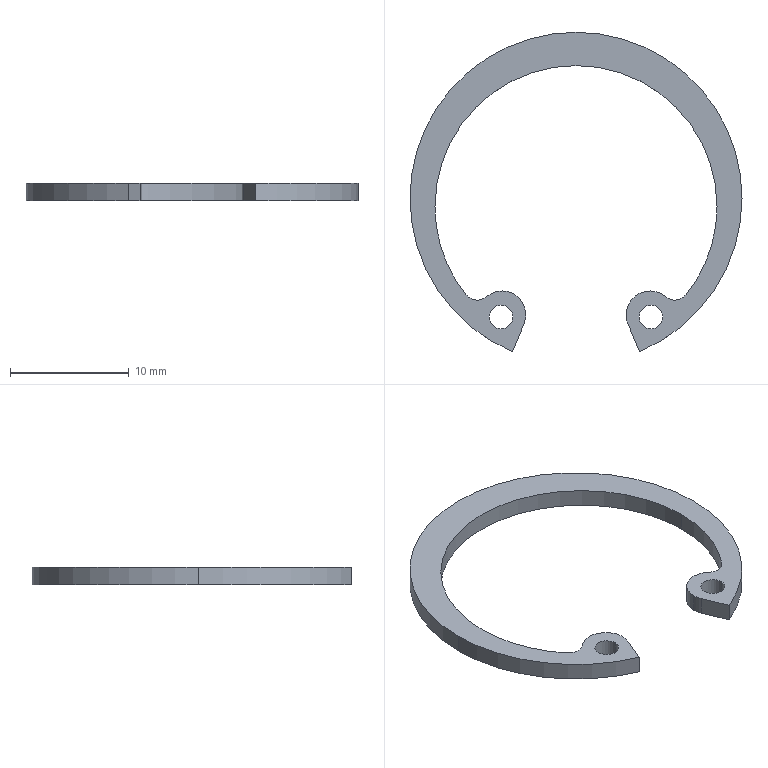Part | SolidWorks | features Extrusion 1 | 1 solid | 19 faces | box 27.9 x 26.838 x 1.5 mm | volume 253.572 mm3 | cylinder 15 | plane 4 | commonest cylinder face diameters 2 x4 4 x3 23.7 x3 27.9 x3 2.4 x2
STEP:
#1=CARTESIAN_POINT('',(5.298,-9.979,1.5));
#2=VERTEX_POINT('',#1);
#3=CARTESIAN_POINT('',(7.298,-9.979,1.5));
#4=VERTEX_POINT('',#3);
#5=CARTESIAN_POINT('',(6.298,-9.979,1.5));
#6=DIRECTION('',(0.,0.,1.));
#7=DIRECTION('',(-1.,0.,0.));
#8=AXIS2_PLACEMENT_3D('',#5,#6,#7);
#9=CIRCLE('',#8,1.);
#10=EDGE_CURVE('',#2,#4,#9,.T.);
#11=ORIENTED_EDGE('',*,*,#10,.T.);
#12=CARTESIAN_POINT('',(7.298,-9.979,0.));
#13=VERTEX_POINT('',#12);
#14=CARTESIAN_POINT('',(7.298,-9.979,1.5));
#15=DIRECTION('',(0.,0.,-1.));
#16=VECTOR('',#15,1000.);
#17=LINE('',#14,#16);
#18=EDGE_CURVE('',#4,#13,#17,.T.);
#19=ORIENTED_EDGE('',*,*,#18,.T.);
#20=CARTESIAN_POINT('',(5.298,-9.979,0.));
#21=VERTEX_POINT('',#20);
#22=CARTESIAN_POINT('',(6.298,-9.979,0.));
#23=DIRECTION('',(0.,0.,1.));
#24=DIRECTION('',(-1.,0.,0.));
#25=AXIS2_PLACEMENT_3D('',#22,#23,#24);
#26=CIRCLE('',#25,1.);
#27=EDGE_CURVE('',#21,#13,#26,.T.);
#28=ORIENTED_EDGE('',*,*,#27,.F.);
#29=CARTESIAN_POINT('',(5.298,-9.979,1.5));
#30=DIRECTION('',(0.,0.,-1.));
#31=VECTOR('',#30,1000.);
#32=LINE('',#29,#31);
#33=EDGE_CURVE('',#2,#21,#32,.T.);
#34=ORIENTED_EDGE('',*,*,#33,.F.);
#35=EDGE_LOOP('',(#11,#19,#28,#34));
#36=FACE_OUTER_BOUND('',#35,.T.);
#37=CARTESIAN_POINT('',(6.298,-9.979,1.5));
#38=DIRECTION('',(0.,0.,-1.));
#39=DIRECTION('',(-1.,0.,0.));
#40=AXIS2_PLACEMENT_3D('',#37,#38,#39);
#41=CYLINDRICAL_SURFACE('',#40,1.);
#42=ADVANCED_FACE('',(#36),#41,.F.);
#43=CARTESIAN_POINT('',(-7.298,-9.979,1.5));
#44=VERTEX_POINT('',#43);
#45=CARTESIAN_POINT('',(-5.298,-9.979,1.5));
#46=VERTEX_POINT('',#45);
#47=CARTESIAN_POINT('',(-6.298,-9.979,1.5));
#48=DIRECTION('',(0.,0.,1.));
#49=DIRECTION('',(1.,0.,0.));
#50=AXIS2_PLACEMENT_3D('',#47,#48,#49);
#51=CIRCLE('',#50,1.);
#52=EDGE_CURVE('',#44,#46,#51,.T.);
#53=ORIENTED_EDGE('',*,*,#52,.T.);
#54=CARTESIAN_POINT('',(-5.298,-9.979,0.));
#55=VERTEX_POINT('',#54);
#56=CARTESIAN_POINT('',(-5.298,-9.979,1.5));
#57=DIRECTION('',(0.,0.,-1.));
#58=VECTOR('',#57,1000.);
#59=LINE('',#56,#58);
#60=EDGE_CURVE('',#46,#55,#59,.T.);
#61=ORIENTED_EDGE('',*,*,#60,.T.);
#62=CARTESIAN_POINT('',(-7.298,-9.979,0.));
#63=VERTEX_POINT('',#62);
#64=CARTESIAN_POINT('',(-6.298,-9.979,0.));
#65=DIRECTION('',(0.,0.,1.));
#66=DIRECTION('',(1.,0.,0.));
#67=AXIS2_PLACEMENT_3D('',#64,#65,#66);
#68=CIRCLE('',#67,1.);
#69=EDGE_CURVE('',#63,#55,#68,.T.);
#70=ORIENTED_EDGE('',*,*,#69,.F.);
#71=CARTESIAN_POINT('',(-7.298,-9.979,1.5));
#72=DIRECTION('',(0.,0.,-1.));
#73=VECTOR('',#72,1000.);
#74=LINE('',#71,#73);
#75=EDGE_CURVE('',#44,#63,#74,.T.);
#76=ORIENTED_EDGE('',*,*,#75,.F.);
#77=EDGE_LOOP('',(#53,#61,#70,#76));
#78=FACE_OUTER_BOUND('',#77,.T.);
#79=CARTESIAN_POINT('',(-6.298,-9.979,1.5));
#80=DIRECTION('',(0.,0.,-1.));
#81=DIRECTION('',(-1.,0.,0.));
#82=AXIS2_PLACEMENT_3D('',#79,#80,#81);
#83=CYLINDRICAL_SURFACE('',#82,1.);
#84=ADVANCED_FACE('',(#78),#83,.F.);
#85=CARTESIAN_POINT('',(13.95,0.,1.5));
#86=VERTEX_POINT('',#85);
#87=CARTESIAN_POINT('',(-13.95,0.,1.5));
#88=VERTEX_POINT('',#87);
#89=CARTESIAN_POINT('',(0.,0.,1.5));
#90=DIRECTION('',(0.,0.,1.));
#91=DIRECTION('',(1.,0.,0.));
#92=AXIS2_PLACEMENT_3D('',#89,#90,#91);
#93=CIRCLE('',#92,13.95);
#94=EDGE_CURVE('',#86,#88,#93,.T.);
#95=ORIENTED_EDGE('',*,*,#94,.F.);
#96=CARTESIAN_POINT('',(13.95,0.,0.));
#97=VERTEX_POINT('',#96);
#98=CARTESIAN_POINT('',(13.95,0.,1.5));
#99=DIRECTION('',(0.,0.,-1.));
#100=VECTOR('',#99,1000.);
#101=LINE('',#98,#100);
#102=EDGE_CURVE('',#86,#97,#101,.T.);
#103=ORIENTED_EDGE('',*,*,#102,.T.);
#104=CARTESIAN_POINT('',(-13.95,0.,0.));
#105=VERTEX_POINT('',#104);
#106=CARTESIAN_POINT('',(0.,0.,0.));
#107=DIRECTION('',(0.,0.,1.));
#108=DIRECTION('',(1.,0.,0.));
#109=AXIS2_PLACEMENT_3D('',#106,#107,#108);
#110=CIRCLE('',#109,13.95);
#111=EDGE_CURVE('',#97,#105,#110,.T.);
#112=ORIENTED_EDGE('',*,*,#111,.T.);
#113=CARTESIAN_POINT('',(-13.95,0.,1.5));
#114=DIRECTION('',(0.,0.,-1.));
#115=VECTOR('',#114,1000.);
#116=LINE('',#113,#115);
#117=EDGE_CURVE('',#88,#105,#116,.T.);
#118=ORIENTED_EDGE('',*,*,#117,.F.);
#119=EDGE_LOOP('',(#95,#103,#112,#118));
#120=FACE_OUTER_BOUND('',#119,.T.);
#121=CARTESIAN_POINT('',(0.,0.,1.5));
#122=DIRECTION('',(0.,0.,-1.));
#123=DIRECTION('',(-1.,0.,0.));
#124=AXIS2_PLACEMENT_3D('',#121,#122,#123);
#125=CYLINDRICAL_SURFACE('',#124,13.95);
#126=ADVANCED_FACE('',(#120),#125,.T.);
#127=CARTESIAN_POINT('',(-5.338,-12.888,1.5));
#128=VERTEX_POINT('',#127);
#129=CARTESIAN_POINT('',(0.,0.,1.5));
#130=DIRECTION('',(0.,0.,1.));
#131=DIRECTION('',(1.,0.,0.));
#132=AXIS2_PLACEMENT_3D('',#129,#130,#131);
#133=CIRCLE('',#132,13.95);
#134=EDGE_CURVE('',#88,#128,#133,.T.);
#135=ORIENTED_EDGE('',*,*,#134,.F.);
#136=ORIENTED_EDGE('',*,*,#117,.T.);
#137=CARTESIAN_POINT('',(-5.338,-12.888,0.));
#138=VERTEX_POINT('',#137);
#139=CARTESIAN_POINT('',(0.,0.,0.));
#140=DIRECTION('',(0.,0.,1.));
#141=DIRECTION('',(1.,0.,0.));
#142=AXIS2_PLACEMENT_3D('',#139,#140,#141);
#143=CIRCLE('',#142,13.95);
#144=EDGE_CURVE('',#105,#138,#143,.T.);
#145=ORIENTED_EDGE('',*,*,#144,.T.);
#146=CARTESIAN_POINT('',(-5.338,-12.888,1.5));
#147=DIRECTION('',(0.,0.,-1.));
#148=VECTOR('',#147,1000.);
#149=LINE('',#146,#148);
#150=EDGE_CURVE('',#128,#138,#149,.T.);
#151=ORIENTED_EDGE('',*,*,#150,.F.);
#152=EDGE_LOOP('',(#135,#136,#145,#151));
#153=FACE_OUTER_BOUND('',#152,.T.);
#154=CARTESIAN_POINT('',(0.,0.,1.5));
#155=DIRECTION('',(0.,0.,-1.));
#156=DIRECTION('',(-1.,0.,0.));
#157=AXIS2_PLACEMENT_3D('',#154,#155,#156);
#158=CYLINDRICAL_SURFACE('',#157,13.95);
#159=ADVANCED_FACE('',(#153),#158,.T.);
#160=CARTESIAN_POINT('',(4.217,-9.782,1.5));
#161=VERTEX_POINT('',#160);
#162=CARTESIAN_POINT('',(4.369,-10.547,1.5));
#163=VERTEX_POINT('',#162);
#164=CARTESIAN_POINT('',(6.217,-9.782,1.5));
#165=DIRECTION('',(0.,0.,1.));
#166=DIRECTION('',(-1.,0.,0.));
#167=AXIS2_PLACEMENT_3D('',#164,#165,#166);
#168=CIRCLE('',#167,2.);
#169=EDGE_CURVE('',#161,#163,#168,.T.);
#170=ORIENTED_EDGE('',*,*,#169,.F.);
#171=CARTESIAN_POINT('',(4.217,-9.782,0.));
#172=VERTEX_POINT('',#171);
#173=CARTESIAN_POINT('',(4.217,-9.782,1.5));
#174=DIRECTION('',(0.,0.,-1.));
#175=VECTOR('',#174,1000.);
#176=LINE('',#173,#175);
#177=EDGE_CURVE('',#161,#172,#176,.T.);
#178=ORIENTED_EDGE('',*,*,#177,.T.);
#179=CARTESIAN_POINT('',(4.369,-10.547,0.));
#180=VERTEX_POINT('',#179);
#181=CARTESIAN_POINT('',(6.217,-9.782,0.));
#182=DIRECTION('',(0.,0.,1.));
#183=DIRECTION('',(-1.,0.,0.));
#184=AXIS2_PLACEMENT_3D('',#181,#182,#183);
#185=CIRCLE('',#184,2.);
#186=EDGE_CURVE('',#172,#180,#185,.T.);
#187=ORIENTED_EDGE('',*,*,#186,.T.);
#188=CARTESIAN_POINT('',(4.369,-10.547,1.5));
#189=DIRECTION('',(0.,0.,-1.));
#190=VECTOR('',#189,1000.);
#191=LINE('',#188,#190);
#192=EDGE_CURVE('',#163,#180,#191,.T.);
#193=ORIENTED_EDGE('',*,*,#192,.F.);
#194=EDGE_LOOP('',(#170,#178,#187,#193));
#195=FACE_OUTER_BOUND('',#194,.T.);
#196=CARTESIAN_POINT('',(6.217,-9.782,1.5));
#197=DIRECTION('',(0.,0.,-1.));
#198=DIRECTION('',(-1.,0.,0.));
#199=AXIS2_PLACEMENT_3D('',#196,#197,#198);
#200=CYLINDRICAL_SURFACE('',#199,2.);
#201=ADVANCED_FACE('',(#195),#200,.T.);
#202=CARTESIAN_POINT('',(11.85,-0.7,1.5));
#203=VERTEX_POINT('',#202);
#204=CARTESIAN_POINT('',(9.246,-8.112,1.5));
#205=VERTEX_POINT('',#204);
#206=CARTESIAN_POINT('',(0.,-0.7,1.5));
#207=DIRECTION('',(0.,0.,-1.));
#208=DIRECTION('',(1.,0.,0.));
#209=AXIS2_PLACEMENT_3D('',#206,#207,#208);
#210=CIRCLE('',#209,11.85);
#211=EDGE_CURVE('',#203,#205,#210,.T.);
#212=ORIENTED_EDGE('',*,*,#211,.F.);
#213=CARTESIAN_POINT('',(11.85,-0.7,0.));
#214=VERTEX_POINT('',#213);
#215=CARTESIAN_POINT('',(11.85,-0.7,1.5));
#216=DIRECTION('',(0.,0.,-1.));
#217=VECTOR('',#216,1000.);
#218=LINE('',#215,#217);
#219=EDGE_CURVE('',#203,#214,#218,.T.);
#220=ORIENTED_EDGE('',*,*,#219,.T.);
#221=CARTESIAN_POINT('',(9.246,-8.112,0.));
#222=VERTEX_POINT('',#221);
#223=CARTESIAN_POINT('',(0.,-0.7,0.));
#224=DIRECTION('',(0.,0.,-1.));
#225=DIRECTION('',(1.,0.,0.));
#226=AXIS2_PLACEMENT_3D('',#223,#224,#225);
#227=CIRCLE('',#226,11.85);
#228=EDGE_CURVE('',#214,#222,#227,.T.);
#229=ORIENTED_EDGE('',*,*,#228,.T.);
#230=CARTESIAN_POINT('',(9.246,-8.112,1.5));
#231=DIRECTION('',(0.,0.,-1.));
#232=VECTOR('',#231,1000.);
#233=LINE('',#230,#232);
#234=EDGE_CURVE('',#205,#222,#233,.T.);
#235=ORIENTED_EDGE('',*,*,#234,.F.);
#236=EDGE_LOOP('',(#212,#220,#229,#235));
#237=FACE_OUTER_BOUND('',#236,.T.);
#238=CARTESIAN_POINT('',(0.,-0.7,1.5));
#239=DIRECTION('',(0.,0.,-1.));
#240=DIRECTION('',(-1.,0.,0.));
#241=AXIS2_PLACEMENT_3D('',#238,#239,#240);
#242=CYLINDRICAL_SURFACE('',#241,11.85);
#243=ADVANCED_FACE('',(#237),#242,.F.);
#244=ORIENTED_EDGE('',*,*,#219,.F.);
#245=CARTESIAN_POINT('',(-11.85,-0.7,1.5));
#246=VERTEX_POINT('',#245);
#247=CARTESIAN_POINT('',(0.,-0.7,1.5));
#248=DIRECTION('',(0.,0.,-1.));
#249=DIRECTION('',(1.,0.,0.));
#250=AXIS2_PLACEMENT_3D('',#247,#248,#249);
#251=CIRCLE('',#250,11.85);
#252=EDGE_CURVE('',#246,#203,#251,.T.);
#253=ORIENTED_EDGE('',*,*,#252,.F.);
#254=CARTESIAN_POINT('',(-11.85,-0.7,0.));
#255=VERTEX_POINT('',#254);
#256=CARTESIAN_POINT('',(-11.85,-0.7,1.5));
#257=DIRECTION('',(0.,0.,-1.));
#258=VECTOR('',#257,1000.);
#259=LINE('',#256,#258);
#260=EDGE_CURVE('',#246,#255,#259,.T.);
#261=ORIENTED_EDGE('',*,*,#260,.T.);
#262=CARTESIAN_POINT('',(0.,-0.7,0.));
#263=DIRECTION('',(0.,0.,-1.));
#264=DIRECTION('',(1.,0.,0.));
#265=AXIS2_PLACEMENT_3D('',#262,#263,#264);
#266=CIRCLE('',#265,11.85);
#267=EDGE_CURVE('',#255,#214,#266,.T.);
#268=ORIENTED_EDGE('',*,*,#267,.T.);
#269=EDGE_LOOP('',(#244,#253,#261,#268));
#270=FACE_OUTER_BOUND('',#269,.T.);
#271=CARTESIAN_POINT('',(0.,-0.7,1.5));
#272=DIRECTION('',(0.,0.,-1.));
#273=DIRECTION('',(-1.,0.,0.));
#274=AXIS2_PLACEMENT_3D('',#271,#272,#273);
#275=CYLINDRICAL_SURFACE('',#274,11.85);
#276=ADVANCED_FACE('',(#270),#275,.F.);
#277=ORIENTED_EDGE('',*,*,#52,.F.);
#278=CARTESIAN_POINT('',(-6.298,-9.979,1.5));
#279=DIRECTION('',(0.,0.,1.));
#280=DIRECTION('',(1.,0.,0.));
#281=AXIS2_PLACEMENT_3D('',#278,#279,#280);
#282=CIRCLE('',#281,1.);
#283=EDGE_CURVE('',#46,#44,#282,.T.);
#284=ORIENTED_EDGE('',*,*,#283,.F.);
#285=EDGE_LOOP('',(#277,#284));
#286=FACE_BOUND('',#285,.T.);
#287=CARTESIAN_POINT('',(-4.369,-10.547,1.5));
#288=VERTEX_POINT('',#287);
#289=CARTESIAN_POINT('',(-7.525,-8.269,1.5));
#290=VERTEX_POINT('',#289);
#291=CARTESIAN_POINT('',(-6.217,-9.782,1.5));
#292=DIRECTION('',(0.,0.,1.));
#293=DIRECTION('',(1.,0.,0.));
#294=AXIS2_PLACEMENT_3D('',#291,#292,#293);
#295=CIRCLE('',#294,2.);
#296=EDGE_CURVE('',#288,#290,#295,.T.);
#297=ORIENTED_EDGE('',*,*,#296,.T.);
#298=CARTESIAN_POINT('',(-9.246,-8.112,1.5));
#299=VERTEX_POINT('',#298);
#300=CARTESIAN_POINT('',(-8.31,-7.361,1.5));
#301=DIRECTION('',(0.,0.,-1.));
#302=DIRECTION('',(-1.,0.,0.));
#303=AXIS2_PLACEMENT_3D('',#300,#301,#302);
#304=CIRCLE('',#303,1.2);
#305=EDGE_CURVE('',#290,#299,#304,.T.);
#306=ORIENTED_EDGE('',*,*,#305,.T.);
#307=CARTESIAN_POINT('',(0.,-0.7,1.5));
#308=DIRECTION('',(0.,0.,-1.));
#309=DIRECTION('',(1.,0.,0.));
#310=AXIS2_PLACEMENT_3D('',#307,#308,#309);
#311=CIRCLE('',#310,11.85);
#312=EDGE_CURVE('',#299,#246,#311,.T.);
#313=ORIENTED_EDGE('',*,*,#312,.T.);
#314=ORIENTED_EDGE('',*,*,#252,.T.);
#315=ORIENTED_EDGE('',*,*,#211,.T.);
#316=CARTESIAN_POINT('',(7.525,-8.269,1.5));
#317=VERTEX_POINT('',#316);
#318=CARTESIAN_POINT('',(8.31,-7.361,1.5));
#319=DIRECTION('',(0.,0.,-1.));
#320=DIRECTION('',(1.,0.,0.));
#321=AXIS2_PLACEMENT_3D('',#318,#319,#320);
#322=CIRCLE('',#321,1.2);
#323=EDGE_CURVE('',#205,#317,#322,.T.);
#324=ORIENTED_EDGE('',*,*,#323,.T.);
#325=CARTESIAN_POINT('',(6.217,-9.782,1.5));
#326=DIRECTION('',(0.,0.,1.));
#327=DIRECTION('',(-1.,0.,0.));
#328=AXIS2_PLACEMENT_3D('',#325,#326,#327);
#329=CIRCLE('',#328,2.);
#330=EDGE_CURVE('',#317,#161,#329,.T.);
#331=ORIENTED_EDGE('',*,*,#330,.T.);
#332=ORIENTED_EDGE('',*,*,#169,.T.);
#333=CARTESIAN_POINT('',(5.338,-12.888,1.5));
#334=VERTEX_POINT('',#333);
#335=CARTESIAN_POINT('',(4.369,-10.547,1.5));
#336=DIRECTION('',(0.3827,-0.9239,0.));
#337=VECTOR('',#336,1000.);
#338=LINE('',#335,#337);
#339=EDGE_CURVE('',#163,#334,#338,.T.);
#340=ORIENTED_EDGE('',*,*,#339,.T.);
#341=CARTESIAN_POINT('',(0.,0.,1.5));
#342=DIRECTION('',(0.,0.,1.));
#343=DIRECTION('',(1.,0.,0.));
#344=AXIS2_PLACEMENT_3D('',#341,#342,#343);
#345=CIRCLE('',#344,13.95);
#346=EDGE_CURVE('',#334,#86,#345,.T.);
#347=ORIENTED_EDGE('',*,*,#346,.T.);
#348=ORIENTED_EDGE('',*,*,#94,.T.);
#349=ORIENTED_EDGE('',*,*,#134,.T.);
#350=CARTESIAN_POINT('',(-4.369,-10.547,1.5));
#351=DIRECTION('',(0.3827,0.9239,0.));
#352=VECTOR('',#351,1000.);
#353=LINE('',#350,#352);
#354=EDGE_CURVE('',#128,#288,#353,.T.);
#355=ORIENTED_EDGE('',*,*,#354,.T.);
#356=EDGE_LOOP('',(#297,#306,#313,#314,#315,#324,#331,#332,#340,#347,#348,#349,#355));
#357=FACE_OUTER_BOUND('',#356,.T.);
#358=ORIENTED_EDGE('',*,*,#10,.F.);
#359=CARTESIAN_POINT('',(6.298,-9.979,1.5));
#360=DIRECTION('',(0.,0.,1.));
#361=DIRECTION('',(-1.,0.,0.));
#362=AXIS2_PLACEMENT_3D('',#359,#360,#361);
#363=CIRCLE('',#362,1.);
#364=EDGE_CURVE('',#4,#2,#363,.T.);
#365=ORIENTED_EDGE('',*,*,#364,.F.);
#366=EDGE_LOOP('',(#358,#365));
#367=FACE_BOUND('',#366,.T.);
#368=CARTESIAN_POINT('',(-6.217,-9.782,1.5));
#369=DIRECTION('',(0.,0.,1.));
#370=DIRECTION('',(1.,0.,0.));
#371=AXIS2_PLACEMENT_3D('',#368,#369,#370);
#372=PLANE('',#371);
#373=ADVANCED_FACE('',(#286,#357,#367),#372,.T.);
#374=CARTESIAN_POINT('',(-4.369,-10.547,0.));
#375=VERTEX_POINT('',#374);
#376=CARTESIAN_POINT('',(-7.525,-8.269,0.));
#377=VERTEX_POINT('',#376);
#378=CARTESIAN_POINT('',(-6.217,-9.782,0.));
#379=DIRECTION('',(0.,0.,1.));
#380=DIRECTION('',(1.,0.,0.));
#381=AXIS2_PLACEMENT_3D('',#378,#379,#380);
#382=CIRCLE('',#381,2.);
#383=EDGE_CURVE('',#375,#377,#382,.T.);
#384=ORIENTED_EDGE('',*,*,#383,.F.);
#385=CARTESIAN_POINT('',(-4.369,-10.547,0.));
#386=DIRECTION('',(0.3827,0.9239,0.));
#387=VECTOR('',#386,1000.);
#388=LINE('',#385,#387);
#389=EDGE_CURVE('',#138,#375,#388,.T.);
#390=ORIENTED_EDGE('',*,*,#389,.F.);
#391=ORIENTED_EDGE('',*,*,#144,.F.);
#392=ORIENTED_EDGE('',*,*,#111,.F.);
#393=CARTESIAN_POINT('',(5.338,-12.888,0.));
#394=VERTEX_POINT('',#393);
#395=CARTESIAN_POINT('',(0.,0.,0.));
#396=DIRECTION('',(0.,0.,1.));
#397=DIRECTION('',(1.,0.,0.));
#398=AXIS2_PLACEMENT_3D('',#395,#396,#397);
#399=CIRCLE('',#398,13.95);
#400=EDGE_CURVE('',#394,#97,#399,.T.);
#401=ORIENTED_EDGE('',*,*,#400,.F.);
#402=CARTESIAN_POINT('',(4.369,-10.547,0.));
#403=DIRECTION('',(0.3827,-0.9239,0.));
#404=VECTOR('',#403,1000.);
#405=LINE('',#402,#404);
#406=EDGE_CURVE('',#180,#394,#405,.T.);
#407=ORIENTED_EDGE('',*,*,#406,.F.);
#408=ORIENTED_EDGE('',*,*,#186,.F.);
#409=CARTESIAN_POINT('',(7.525,-8.269,0.));
#410=VERTEX_POINT('',#409);
#411=CARTESIAN_POINT('',(6.217,-9.782,0.));
#412=DIRECTION('',(0.,0.,1.));
#413=DIRECTION('',(-1.,0.,0.));
#414=AXIS2_PLACEMENT_3D('',#411,#412,#413);
#415=CIRCLE('',#414,2.);
#416=EDGE_CURVE('',#410,#172,#415,.T.);
#417=ORIENTED_EDGE('',*,*,#416,.F.);
#418=CARTESIAN_POINT('',(8.31,-7.361,0.));
#419=DIRECTION('',(0.,0.,-1.));
#420=DIRECTION('',(1.,0.,0.));
#421=AXIS2_PLACEMENT_3D('',#418,#419,#420);
#422=CIRCLE('',#421,1.2);
#423=EDGE_CURVE('',#222,#410,#422,.T.);
#424=ORIENTED_EDGE('',*,*,#423,.F.);
#425=ORIENTED_EDGE('',*,*,#228,.F.);
#426=ORIENTED_EDGE('',*,*,#267,.F.);
#427=CARTESIAN_POINT('',(-9.246,-8.112,0.));
#428=VERTEX_POINT('',#427);
#429=CARTESIAN_POINT('',(0.,-0.7,0.));
#430=DIRECTION('',(0.,0.,-1.));
#431=DIRECTION('',(1.,0.,0.));
#432=AXIS2_PLACEMENT_3D('',#429,#430,#431);
#433=CIRCLE('',#432,11.85);
#434=EDGE_CURVE('',#428,#255,#433,.T.);
#435=ORIENTED_EDGE('',*,*,#434,.F.);
#436=CARTESIAN_POINT('',(-8.31,-7.361,0.));
#437=DIRECTION('',(0.,0.,-1.));
#438=DIRECTION('',(-1.,0.,0.));
#439=AXIS2_PLACEMENT_3D('',#436,#437,#438);
#440=CIRCLE('',#439,1.2);
#441=EDGE_CURVE('',#377,#428,#440,.T.);
#442=ORIENTED_EDGE('',*,*,#441,.F.);
#443=EDGE_LOOP('',(#384,#390,#391,#392,#401,#407,#408,#417,#424,#425,#426,#435,#442));
#444=FACE_OUTER_BOUND('',#443,.T.);
#445=ORIENTED_EDGE('',*,*,#69,.T.);
#446=CARTESIAN_POINT('',(-6.298,-9.979,0.));
#447=DIRECTION('',(0.,0.,1.));
#448=DIRECTION('',(1.,0.,0.));
#449=AXIS2_PLACEMENT_3D('',#446,#447,#448);
#450=CIRCLE('',#449,1.);
#451=EDGE_CURVE('',#55,#63,#450,.T.);
#452=ORIENTED_EDGE('',*,*,#451,.T.);
#453=EDGE_LOOP('',(#445,#452));
#454=FACE_BOUND('',#453,.T.);
#455=ORIENTED_EDGE('',*,*,#27,.T.);
#456=CARTESIAN_POINT('',(6.298,-9.979,0.));
#457=DIRECTION('',(0.,0.,1.));
#458=DIRECTION('',(-1.,0.,0.));
#459=AXIS2_PLACEMENT_3D('',#456,#457,#458);
#460=CIRCLE('',#459,1.);
#461=EDGE_CURVE('',#13,#21,#460,.T.);
#462=ORIENTED_EDGE('',*,*,#461,.T.);
#463=EDGE_LOOP('',(#455,#462));
#464=FACE_BOUND('',#463,.T.);
#465=CARTESIAN_POINT('',(-6.217,-9.782,0.));
#466=DIRECTION('',(0.,0.,1.));
#467=DIRECTION('',(1.,0.,0.));
#468=AXIS2_PLACEMENT_3D('',#465,#466,#467);
#469=PLANE('',#468);
#470=ADVANCED_FACE('',(#444,#454,#464),#469,.F.);
#471=ORIENTED_EDGE('',*,*,#383,.T.);
#472=CARTESIAN_POINT('',(-7.525,-8.269,1.5));
#473=DIRECTION('',(0.,0.,-1.));
#474=VECTOR('',#473,1000.);
#475=LINE('',#472,#474);
#476=EDGE_CURVE('',#290,#377,#475,.T.);
#477=ORIENTED_EDGE('',*,*,#476,.F.);
#478=ORIENTED_EDGE('',*,*,#296,.F.);
#479=CARTESIAN_POINT('',(-4.369,-10.547,1.5));
#480=DIRECTION('',(0.,0.,-1.));
#481=VECTOR('',#480,1000.);
#482=LINE('',#479,#481);
#483=EDGE_CURVE('',#288,#375,#482,.T.);
#484=ORIENTED_EDGE('',*,*,#483,.T.);
#485=EDGE_LOOP('',(#471,#477,#478,#484));
#486=FACE_OUTER_BOUND('',#485,.T.);
#487=CARTESIAN_POINT('',(-6.217,-9.782,1.5));
#488=DIRECTION('',(0.,0.,-1.));
#489=DIRECTION('',(-1.,0.,0.));
#490=AXIS2_PLACEMENT_3D('',#487,#488,#489);
#491=CYLINDRICAL_SURFACE('',#490,2.);
#492=ADVANCED_FACE('',(#486),#491,.T.);
#493=ORIENTED_EDGE('',*,*,#441,.T.);
#494=CARTESIAN_POINT('',(-9.246,-8.112,1.5));
#495=DIRECTION('',(0.,0.,-1.));
#496=VECTOR('',#495,1000.);
#497=LINE('',#494,#496);
#498=EDGE_CURVE('',#299,#428,#497,.T.);
#499=ORIENTED_EDGE('',*,*,#498,.F.);
#500=ORIENTED_EDGE('',*,*,#305,.F.);
#501=ORIENTED_EDGE('',*,*,#476,.T.);
#502=EDGE_LOOP('',(#493,#499,#500,#501));
#503=FACE_OUTER_BOUND('',#502,.T.);
#504=CARTESIAN_POINT('',(-8.31,-7.361,1.5));
#505=DIRECTION('',(0.,0.,-1.));
#506=DIRECTION('',(-1.,0.,0.));
#507=AXIS2_PLACEMENT_3D('',#504,#505,#506);
#508=CYLINDRICAL_SURFACE('',#507,1.2);
#509=ADVANCED_FACE('',(#503),#508,.F.);
#510=ORIENTED_EDGE('',*,*,#260,.F.);
#511=ORIENTED_EDGE('',*,*,#312,.F.);
#512=ORIENTED_EDGE('',*,*,#498,.T.);
#513=ORIENTED_EDGE('',*,*,#434,.T.);
#514=EDGE_LOOP('',(#510,#511,#512,#513));
#515=FACE_OUTER_BOUND('',#514,.T.);
#516=CARTESIAN_POINT('',(0.,-0.7,1.5));
#517=DIRECTION('',(0.,0.,-1.));
#518=DIRECTION('',(-1.,0.,0.));
#519=AXIS2_PLACEMENT_3D('',#516,#517,#518);
#520=CYLINDRICAL_SURFACE('',#519,11.85);
#521=ADVANCED_FACE('',(#515),#520,.F.);
#522=ORIENTED_EDGE('',*,*,#423,.T.);
#523=CARTESIAN_POINT('',(7.525,-8.269,1.5));
#524=DIRECTION('',(0.,0.,-1.));
#525=VECTOR('',#524,1000.);
#526=LINE('',#523,#525);
#527=EDGE_CURVE('',#317,#410,#526,.T.);
#528=ORIENTED_EDGE('',*,*,#527,.F.);
#529=ORIENTED_EDGE('',*,*,#323,.F.);
#530=ORIENTED_EDGE('',*,*,#234,.T.);
#531=EDGE_LOOP('',(#522,#528,#529,#530));
#532=FACE_OUTER_BOUND('',#531,.T.);
#533=CARTESIAN_POINT('',(8.31,-7.361,1.5));
#534=DIRECTION('',(0.,0.,-1.));
#535=DIRECTION('',(-1.,0.,0.));
#536=AXIS2_PLACEMENT_3D('',#533,#534,#535);
#537=CYLINDRICAL_SURFACE('',#536,1.2);
#538=ADVANCED_FACE('',(#532),#537,.F.);
#539=ORIENTED_EDGE('',*,*,#177,.F.);
#540=ORIENTED_EDGE('',*,*,#330,.F.);
#541=ORIENTED_EDGE('',*,*,#527,.T.);
#542=ORIENTED_EDGE('',*,*,#416,.T.);
#543=EDGE_LOOP('',(#539,#540,#541,#542));
#544=FACE_OUTER_BOUND('',#543,.T.);
#545=CARTESIAN_POINT('',(6.217,-9.782,1.5));
#546=DIRECTION('',(0.,0.,-1.));
#547=DIRECTION('',(-1.,0.,0.));
#548=AXIS2_PLACEMENT_3D('',#545,#546,#547);
#549=CYLINDRICAL_SURFACE('',#548,2.);
#550=ADVANCED_FACE('',(#544),#549,.T.);
#551=ORIENTED_EDGE('',*,*,#406,.T.);
#552=CARTESIAN_POINT('',(5.338,-12.888,1.5));
#553=DIRECTION('',(0.,0.,-1.));
#554=VECTOR('',#553,1000.);
#555=LINE('',#552,#554);
#556=EDGE_CURVE('',#334,#394,#555,.T.);
#557=ORIENTED_EDGE('',*,*,#556,.F.);
#558=ORIENTED_EDGE('',*,*,#339,.F.);
#559=ORIENTED_EDGE('',*,*,#192,.T.);
#560=EDGE_LOOP('',(#551,#557,#558,#559));
#561=FACE_OUTER_BOUND('',#560,.T.);
#562=CARTESIAN_POINT('',(4.369,-10.547,1.5));
#563=DIRECTION('',(0.9239,0.3827,0.));
#564=DIRECTION('',(-0.3827,0.9239,0.));
#565=AXIS2_PLACEMENT_3D('',#562,#563,#564);
#566=PLANE('',#565);
#567=ADVANCED_FACE('',(#561),#566,.F.);
#568=ORIENTED_EDGE('',*,*,#102,.F.);
#569=ORIENTED_EDGE('',*,*,#346,.F.);
#570=ORIENTED_EDGE('',*,*,#556,.T.);
#571=ORIENTED_EDGE('',*,*,#400,.T.);
#572=EDGE_LOOP('',(#568,#569,#570,#571));
#573=FACE_OUTER_BOUND('',#572,.T.);
#574=CARTESIAN_POINT('',(0.,0.,1.5));
#575=DIRECTION('',(0.,0.,-1.));
#576=DIRECTION('',(-1.,0.,0.));
#577=AXIS2_PLACEMENT_3D('',#574,#575,#576);
#578=CYLINDRICAL_SURFACE('',#577,13.95);
#579=ADVANCED_FACE('',(#573),#578,.T.);
#580=ORIENTED_EDGE('',*,*,#389,.T.);
#581=ORIENTED_EDGE('',*,*,#483,.F.);
#582=ORIENTED_EDGE('',*,*,#354,.F.);
#583=ORIENTED_EDGE('',*,*,#150,.T.);
#584=EDGE_LOOP('',(#580,#581,#582,#583));
#585=FACE_OUTER_BOUND('',#584,.T.);
#586=CARTESIAN_POINT('',(-4.369,-10.547,1.5));
#587=DIRECTION('',(-0.9239,0.3827,0.));
#588=DIRECTION('',(-0.3827,-0.9239,0.));
#589=AXIS2_PLACEMENT_3D('',#586,#587,#588);
#590=PLANE('',#589);
#591=ADVANCED_FACE('',(#585),#590,.F.);
#592=ORIENTED_EDGE('',*,*,#60,.F.);
#593=ORIENTED_EDGE('',*,*,#283,.T.);
#594=ORIENTED_EDGE('',*,*,#75,.T.);
#595=ORIENTED_EDGE('',*,*,#451,.F.);
#596=EDGE_LOOP('',(#592,#593,#594,#595));
#597=FACE_OUTER_BOUND('',#596,.T.);
#598=CARTESIAN_POINT('',(-6.298,-9.979,1.5));
#599=DIRECTION('',(0.,0.,-1.));
#600=DIRECTION('',(-1.,0.,0.));
#601=AXIS2_PLACEMENT_3D('',#598,#599,#600);
#602=CYLINDRICAL_SURFACE('',#601,1.);
#603=ADVANCED_FACE('',(#597),#602,.F.);
#604=ORIENTED_EDGE('',*,*,#18,.F.);
#605=ORIENTED_EDGE('',*,*,#364,.T.);
#606=ORIENTED_EDGE('',*,*,#33,.T.);
#607=ORIENTED_EDGE('',*,*,#461,.F.);
#608=EDGE_LOOP('',(#604,#605,#606,#607));
#609=FACE_OUTER_BOUND('',#608,.T.);
#610=CARTESIAN_POINT('',(6.298,-9.979,1.5));
#611=DIRECTION('',(0.,0.,-1.));
#612=DIRECTION('',(-1.,0.,0.));
#613=AXIS2_PLACEMENT_3D('',#610,#611,#612);
#614=CYLINDRICAL_SURFACE('',#613,1.);
#615=ADVANCED_FACE('',(#609),#614,.F.);
#616=CLOSED_SHELL('',(#42,#84,#126,#159,#201,#243,#276,#373,#470,#492,#509,#521,#538,#550,#567,#579,#591,#603,#615));
#617=MANIFOLD_SOLID_BREP('',#616);
#618=CARTESIAN_POINT('',(0.,0.,0.));
#619=DIRECTION('',(0.,0.,1.));
#620=DIRECTION('',(1.,0.,0.));
#621=AXIS2_PLACEMENT_3D('',#618,#619,#620);
#622=(LENGTH_UNIT()NAMED_UNIT(*)SI_UNIT(.MILLI.,.METRE.));
#623=UNCERTAINTY_MEASURE_WITH_UNIT(LENGTH_MEASURE(0.00001),#622,'','');
#624=(NAMED_UNIT(*)PLANE_ANGLE_UNIT()SI_UNIT($,.RADIAN.));
#625=(NAMED_UNIT(*)SI_UNIT($,.STERADIAN.)SOLID_ANGLE_UNIT());
#626=(GEOMETRIC_REPRESENTATION_CONTEXT(3)GLOBAL_UNCERTAINTY_ASSIGNED_CONTEXT((#623))GLOBAL_UNIT_ASSIGNED_CONTEXT((#622,#624,#625))REPRESENTATION_CONTEXT('',''));
#627=ADVANCED_BREP_SHAPE_REPRESENTATION('',(#617,#621),#626);